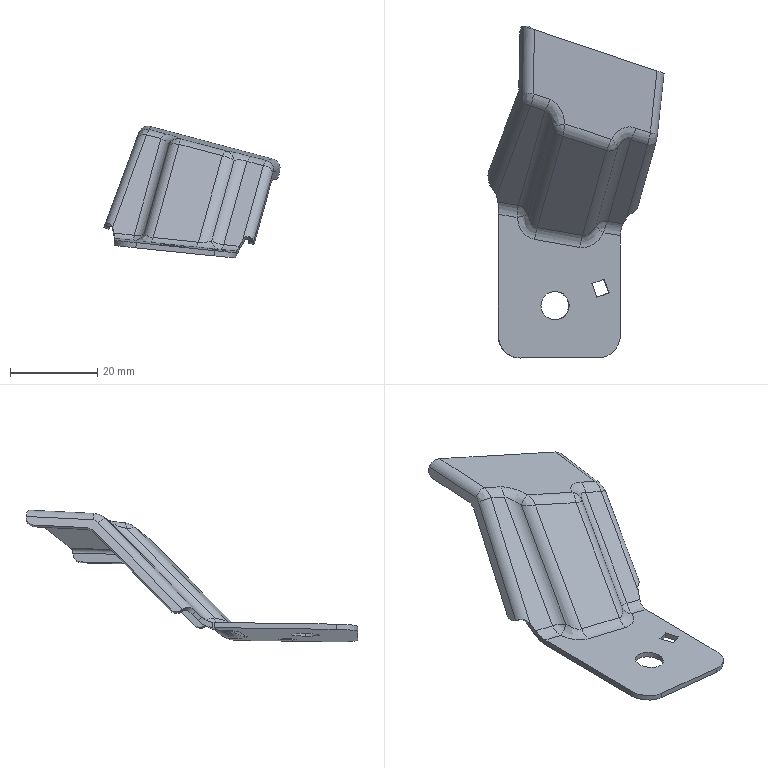Part | 1 solid | 98 faces | box 40.356 x 76.075 x 30.166 mm | volume 3240 mm3 | spline 40 | cylinder 37 | plane 19 | other 2 | commonest cylinder face diameters 6 x6 4 x3 5.453 x3 7.839 x3 7.853 x3 10.239 x3